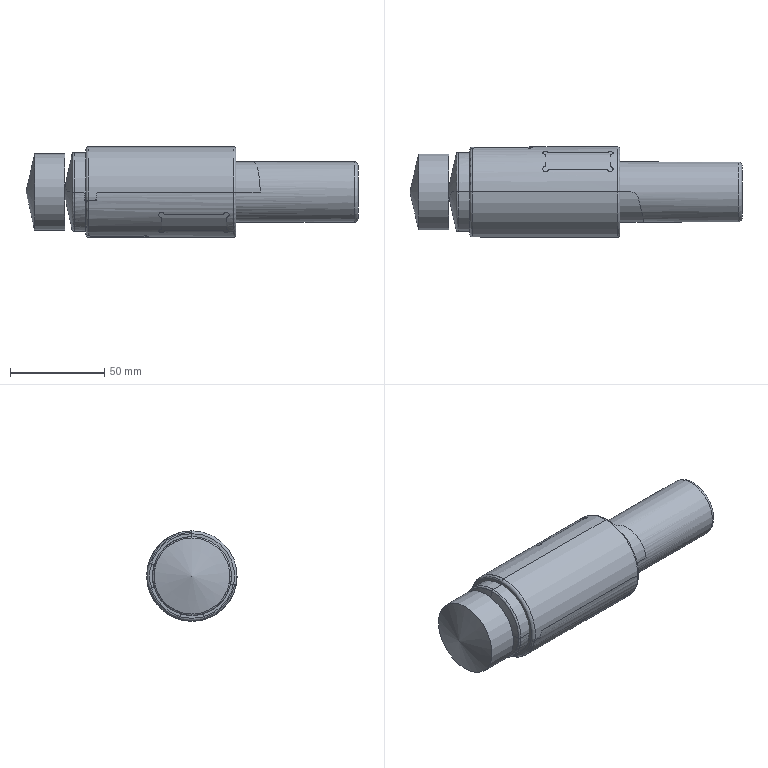CAM job | NX | 3-axis milling, drilling | part box 176.413 x 48 x 48 mm
Tools:
number,name,description,diameter,corner_radius,flute_length,length,flutes
1,ZXZ,Milling Tool-5 Parameters,6.0,0.0,50.0,75.0,2
16,D16R0.8,Milling Tool-5 Parameters,16.0,0.8,50.0,75.0,2
10,D10,Milling Tool-5 Parameters,10.0,0.0,50.0,75.0,2
6,D6,Milling Tool-5 Parameters,6.0,0.0,50.0,75.0,2
8,D6JING,Milling Tool-5 Parameters,6.0,0.0,50.0,75.0,2
2,D2,Milling Tool-5 Parameters,2.0,0.0,50.0,75.0,2
5,D4R0.5,Milling Tool-5 Parameters,4.0,0.5,50.0,75.0,2
13,3.3ZT,Drilling Tool,3.3,0.0,35.0,50.0,2
Operations:
program,operation,operation_type,tool,method,geometry_group,spindle_rpm,surface_speed,feed_per_tooth,feed_cut,feed_plunge,cut_length_mm,path_length_mm,cut_time_min,machine_time_min
1-1,FLOOR_WALL,VolumeBased25DMillingOperation,D16R0.8,METHOD,A,2000.0,100.0,0.5,2000.0,1000.0,19432.859,20602.241,10.318,10.435
1-2,ZLEVEL_PROFILE_COPY,ZLevelMilling,D10,METHOD,A,3500.0,109.0,0.2857,2000.0,100.0,568.085,924.324,0.284,0.3197
1-3,ZLEVEL_PROFILE_COPY_COPY,ZLevelMilling,D10,METHOD,A,2500.0,78.0,0.4,2000.0,1000.0,1348.984,1373.35,0.6909,0.6933
1-3,ZLEVEL_PROFILE_COPY_COPY_COPY_1,ZLevelMilling,D10,METHOD,A,2500.0,78.0,0.4,2000.0,1000.0,1348.984,1373.35,0.6909,0.6933
1-3,ZLEVEL_PROFILE_COPY_COPY_COPY_2,ZLevelMilling,D10,METHOD,A,2500.0,78.0,0.4,2000.0,1000.0,1348.984,1373.35,0.6909,0.6933
1-4,ZLEVEL_PROFILE_COPY_COPY_COPY,ZLevelMilling,D6,METHOD,A,3800.0,71.0,0.2105,1600.0,1000.0,2015.33,2037.724,1.271,1.273
1-4,ZLEVEL_PROFILE_COPY_1,ZLevelMilling,D6,METHOD,A,4000.0,75.0,0.1875,1500.0,100.0,2100.725,2359.591,1.401,1.426
1-4,ZLEVEL_PROFILE_COPY_COPY_COPY_COPY,ZLevelMilling,D6,METHOD,A,3800.0,71.0,0.2105,1600.0,1000.0,2015.33,2037.724,1.271,1.273
1-4,ZLEVEL_PROFILE_COPY_1_COPY,ZLevelMilling,D6,METHOD,A,4000.0,75.0,0.1875,1500.0,100.0,2100.725,2359.591,1.401,1.426
1-4,ZLEVEL_PROFILE_COPY_1_COPY_1,ZLevelMilling,D6,METHOD,A,4000.0,75.0,0.1875,1500.0,100.0,1323.192,1385.374,0.8821,0.8883
1-4,ZLEVEL_PROFILE_COPY_COPY_COPY_3,ZLevelMilling,D6,METHOD,A,4000.0,75.0,0.2,1600.0,1000.0,1335.564,2123.853,0.9166,0.9954
1-4,ZLEVEL_PROFILE_COPY_COPY_COPY_3_COPY_1,ZLevelMilling,D6,METHOD,A,4000.0,75.0,0.2,1600.0,1000.0,1335.564,2123.853,0.9166,0.9954
1-4,ZLEVEL_PROFILE_COPY_COPY_COPY_3_COPY_2,ZLevelMilling,D6,METHOD,A,4000.0,75.0,0.2,1600.0,1000.0,1335.564,2123.853,0.9166,0.9954
1-5,FLOOR_WALL_1,VolumeBased25DMillingOperation,D6JING,METHOD,A,6500.0,122.0,0.0769,1000.0,500.0,612.843,807.069,0.6213,0.6407
1-5,FLOOR_WALL_1_COPY,VolumeBased25DMillingOperation,D6JING,METHOD,A,6500.0,122.0,0.0769,1000.0,500.0,167.686,194.755,0.1716,0.1743
1-5,FLOOR_WALL_1_COPY_COPY_1,VolumeBased25DMillingOperation,D6JING,METHOD,A,6500.0,122.0,0.0769,1000.0,500.0,167.686,194.755,0.1716,0.1743
1-5,FLOOR_WALL_1_COPY_COPY_2,VolumeBased25DMillingOperation,D6JING,METHOD,A,6500.0,122.0,0.0769,1000.0,500.0,167.686,194.755,0.1716,0.1743
1-5,FLOOR_WALL_1_COPY_COPY,VolumeBased25DMillingOperation,D6JING,METHOD,A,6500.0,122.0,0.0769,1000.0,500.0,142.656,165.818,0.1466,0.1489
1-5,FLOOR_WALL_1_COPY_COPY_COPY,VolumeBased25DMillingOperation,D6JING,METHOD,A,6500.0,122.0,0.0769,1000.0,500.0,142.656,165.818,0.1466,0.1489
1-6,ZLEVEL_PROFILE_COPY_COPY_COPY_3_COPY,ZLevelMilling,D2,METHOD,A,5000.0,31.0,0.1,1000.0,1000.0,5129.161,6901.529,5.129,5.306
1-6,ZLEVEL_PROFILE_COPY_COPY_COPY_3_COPY_COPY_1,ZLevelMilling,D2,METHOD,A,5000.0,31.0,0.1,1000.0,1000.0,5129.161,6901.529,5.129,5.306
1-6,ZLEVEL_PROFILE_COPY_COPY_COPY_3_COPY_COPY_2,ZLevelMilling,D2,METHOD,A,5000.0,31.0,0.1,1000.0,1000.0,5129.161,6901.529,5.129,5.306
1-6,ZLEVEL_PROFILE_COPY_COPY_COPY_3_COPY_COPY,ZLevelMilling,D2,METHOD,A,5000.0,31.0,0.1,1000.0,1000.0,2698.794,4257.562,2.699,2.855
1-6,ZLEVEL_PROFILE_COPY_COPY_COPY_3_COPY_COPY_COPY,ZLevelMilling,D2,METHOD,A,5000.0,31.0,0.1,1000.0,1000.0,2698.794,4257.562,2.699,2.855
1-6,ZLEVEL_PROFILE_COPY_COPY_COPY_3_COPY_COPY_3,ZLevelMilling,D2,METHOD,A,5000.0,31.0,0.1,1000.0,1000.0,1653.527,3063.649,1.653,1.794
1-6,ZLEVEL_PROFILE_COPY_2,ZLevelMilling,D2,METHOD,A,5000.0,31.0,0.12,1200.0,100.0,3496.169,3549.062,2.913,2.919
1-7,ZLEVEL_PROFILE_COPY_2_COPY,ZLevelMilling,D4R0.5,METHOD,A,5500.0,103.0,0.2,2200.0,100.0,30769.816,30899.107,13.986,13.999
1-8,DRILLING_COPY,HoleDrilling,ZXZ,METHOD,A,3000.0,56.0,0.025,150.0,0.0,48.0,528.035,0.16,0.208
1-9,DRILLING_COPY_COPY,HoleDrilling,3.3ZT,METHOD,A,2000.0,20.0,0.025,100.0,0.0,1447.0,1980.142,1.07,1.123
2,ZLEVEL_PROFILE_COPY_2_COPY_1,ZLevelMilling,D2,METHOD,A,5000.0,31.0,0.12,1200.0,100.0,3496.169,3549.062,2.913,2.919
PROGRAM_COPY,ZLEVEL_PROFILE_1,ZLevelMilling,D6JING,METHOD,A,5000.0,94.0,0.1,1000.0,100.0,226.207,396.033,0.2262,0.2432